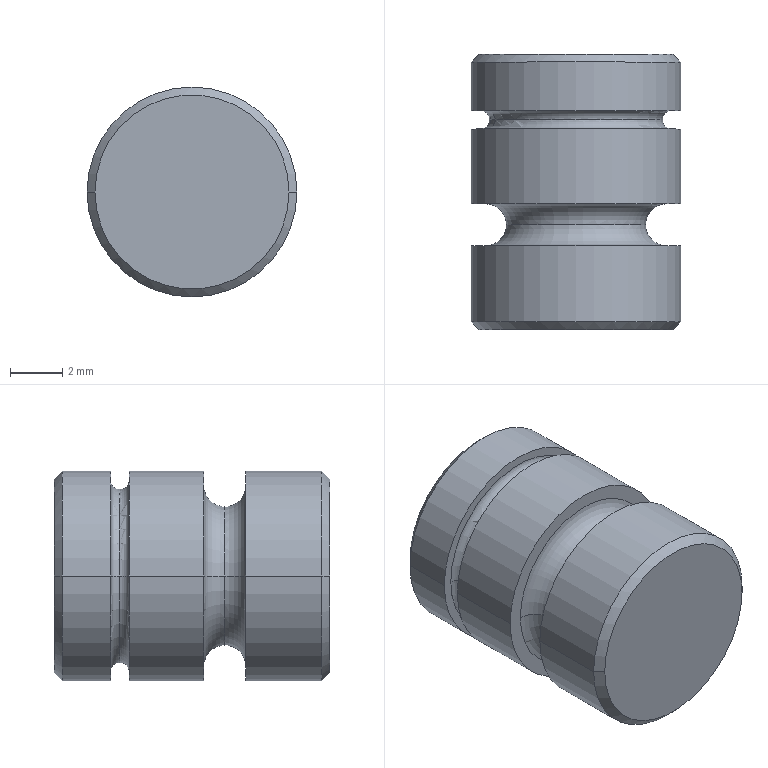Part | Creo | 1 solid | 27 faces | box 8 x 10.5 x 8 mm | volume 445.026 mm3 | cylinder 8 | torus 8 | plane 7 | cone 4 | commonest cylinder face diameters 8 x6 6.2 x2
STEP:
#1=CARTESIAN_POINT('',(0.,0.,0.));
#2=DIRECTION('',(0.,0.,1.));
#3=DIRECTION('',(1.,0.,0.));
#4=AXIS2_PLACEMENT_3D('',#1,#2,#3);
#5=CARTESIAN_POINT('',(59.,47.3,60.91));
#6=VERTEX_POINT('',#5);
#7=CARTESIAN_POINT('',(51.,47.3,60.91));
#8=VERTEX_POINT('',#7);
#9=CARTESIAN_POINT('',(55.,47.3,60.91));
#10=DIRECTION('',(0.,-1.,0.));
#11=DIRECTION('',(1.,0.,0.));
#12=AXIS2_PLACEMENT_3D('',#9,#10,#11);
#13=CIRCLE('',#12,4.);
#14=EDGE_CURVE('',#6,#8,#13,.T.);
#15=ORIENTED_EDGE('',*,*,#14,.T.);
#16=CARTESIAN_POINT('',(51.,50.15,60.91));
#17=VERTEX_POINT('',#16);
#18=CARTESIAN_POINT('',(51.,47.3,60.91));
#19=DIRECTION('',(0.,1.,0.));
#20=VECTOR('',#19,2.85);
#21=LINE('',#18,#20);
#22=EDGE_CURVE('',#8,#17,#21,.T.);
#23=ORIENTED_EDGE('',*,*,#22,.T.);
#24=CARTESIAN_POINT('',(59.,50.15,60.91));
#25=VERTEX_POINT('',#24);
#26=CARTESIAN_POINT('',(55.,50.15,60.91));
#27=DIRECTION('',(0.,1.,0.));
#28=DIRECTION('',(-1.,0.,0.));
#29=AXIS2_PLACEMENT_3D('',#26,#27,#28);
#30=CIRCLE('',#29,4.);
#31=EDGE_CURVE('',#17,#25,#30,.T.);
#32=ORIENTED_EDGE('',*,*,#31,.T.);
#33=CARTESIAN_POINT('',(59.,47.3,60.91));
#34=DIRECTION('',(0.,1.,0.));
#35=VECTOR('',#34,2.85);
#36=LINE('',#33,#35);
#37=EDGE_CURVE('',#6,#25,#36,.T.);
#38=ORIENTED_EDGE('',*,*,#37,.F.);
#39=EDGE_LOOP('',(#15,#23,#32,#38));
#40=FACE_OUTER_BOUND('',#39,.F.);
#41=CARTESIAN_POINT('',(55.,42.5,60.91));
#42=DIRECTION('',(0.,1.,0.));
#43=DIRECTION('',(-1.,0.,0.));
#44=AXIS2_PLACEMENT_3D('',#41,#42,#43);
#45=CYLINDRICAL_SURFACE('',#44,4.);
#46=ADVANCED_FACE('',(#40),#45,.T.);
#47=ORIENTED_EDGE('',*,*,#14,.F.);
#48=CARTESIAN_POINT('',(55.,47.3,60.91));
#49=DIRECTION('',(0.,-1.,0.));
#50=DIRECTION('',(-1.,0.,0.));
#51=AXIS2_PLACEMENT_3D('',#48,#49,#50);
#52=CIRCLE('',#51,4.);
#53=EDGE_CURVE('',#8,#6,#52,.T.);
#54=ORIENTED_EDGE('',*,*,#53,.F.);
#55=EDGE_LOOP('',(#47,#54));
#56=FACE_OUTER_BOUND('',#55,.F.);
#57=CARTESIAN_POINT('',(51.55,47.3,60.91));
#58=VERTEX_POINT('',#57);
#59=CARTESIAN_POINT('',(58.45,47.3,60.91));
#60=VERTEX_POINT('',#59);
#61=CARTESIAN_POINT('',(55.,47.3,60.91));
#62=DIRECTION('',(0.,1.,0.));
#63=DIRECTION('',(-1.,0.,0.));
#64=AXIS2_PLACEMENT_3D('',#61,#62,#63);
#65=CIRCLE('',#64,3.45);
#66=EDGE_CURVE('',#58,#60,#65,.T.);
#67=ORIENTED_EDGE('',*,*,#66,.F.);
#68=CARTESIAN_POINT('',(55.,47.3,60.91));
#69=DIRECTION('',(0.,1.,0.));
#70=DIRECTION('',(1.,0.,0.));
#71=AXIS2_PLACEMENT_3D('',#68,#69,#70);
#72=CIRCLE('',#71,3.45);
#73=EDGE_CURVE('',#60,#58,#72,.T.);
#74=ORIENTED_EDGE('',*,*,#73,.F.);
#75=EDGE_LOOP('',(#67,#74));
#76=FACE_BOUND('',#75,.F.);
#77=CARTESIAN_POINT('',(63.45,47.3,60.91));
#78=DIRECTION('',(0.,-1.,0.));
#79=DIRECTION('',(1.,0.,0.));
#80=AXIS2_PLACEMENT_3D('',#77,#78,#79);
#81=PLANE('',#80);
#82=ADVANCED_FACE('',(#56,#76),#81,.T.);
#83=ORIENTED_EDGE('',*,*,#66,.T.);
#84=CARTESIAN_POINT('',(57.65,46.5,60.91));
#85=VERTEX_POINT('',#84);
#86=CARTESIAN_POINT('',(58.45,46.5,60.91));
#87=DIRECTION('',(0.,0.,1.));
#88=DIRECTION('',(0.,1.,0.));
#89=AXIS2_PLACEMENT_3D('',#86,#87,#88);
#90=CIRCLE('',#89,0.8);
#91=EDGE_CURVE('',#60,#85,#90,.T.);
#92=ORIENTED_EDGE('',*,*,#91,.T.);
#93=CARTESIAN_POINT('',(52.35,46.5,60.91));
#94=VERTEX_POINT('',#93);
#95=CARTESIAN_POINT('',(55.,46.5,60.91));
#96=DIRECTION('',(0.,1.,0.));
#97=DIRECTION('',(-1.,0.,0.));
#98=AXIS2_PLACEMENT_3D('',#95,#96,#97);
#99=CIRCLE('',#98,2.65);
#100=EDGE_CURVE('',#94,#85,#99,.T.);
#101=ORIENTED_EDGE('',*,*,#100,.F.);
#102=CARTESIAN_POINT('',(51.55,46.5,60.91));
#103=DIRECTION('',(0.,0.,-1.));
#104=DIRECTION('',(0.,1.,0.));
#105=AXIS2_PLACEMENT_3D('',#102,#103,#104);
#106=CIRCLE('',#105,0.8);
#107=EDGE_CURVE('',#58,#94,#106,.T.);
#108=ORIENTED_EDGE('',*,*,#107,.F.);
#109=EDGE_LOOP('',(#83,#92,#101,#108));
#110=FACE_OUTER_BOUND('',#109,.F.);
#111=CARTESIAN_POINT('',(55.,46.5,60.91));
#112=DIRECTION('',(0.,1.,0.));
#113=DIRECTION('',(-1.,0.,0.));
#114=AXIS2_PLACEMENT_3D('',#111,#112,#113);
#115=TOROIDAL_SURFACE('',#114,3.45,0.8);
#116=ADVANCED_FACE('',(#110),#115,.F.);
#117=ORIENTED_EDGE('',*,*,#73,.T.);
#118=ORIENTED_EDGE('',*,*,#107,.T.);
#119=CARTESIAN_POINT('',(55.,46.5,60.91));
#120=DIRECTION('',(0.,1.,0.));
#121=DIRECTION('',(1.,0.,0.));
#122=AXIS2_PLACEMENT_3D('',#119,#120,#121);
#123=CIRCLE('',#122,2.65);
#124=EDGE_CURVE('',#85,#94,#123,.T.);
#125=ORIENTED_EDGE('',*,*,#124,.F.);
#126=ORIENTED_EDGE('',*,*,#91,.F.);
#127=EDGE_LOOP('',(#117,#118,#125,#126));
#128=FACE_OUTER_BOUND('',#127,.F.);
#129=CARTESIAN_POINT('',(55.,46.5,60.91));
#130=DIRECTION('',(0.,1.,0.));
#131=DIRECTION('',(-1.,0.,0.));
#132=AXIS2_PLACEMENT_3D('',#129,#130,#131);
#133=TOROIDAL_SURFACE('',#132,3.45,0.8);
#134=ADVANCED_FACE('',(#128),#133,.F.);
#135=CARTESIAN_POINT('',(51.55,45.7,60.91));
#136=VERTEX_POINT('',#135);
#137=CARTESIAN_POINT('',(58.45,45.7,60.91));
#138=VERTEX_POINT('',#137);
#139=CARTESIAN_POINT('',(55.,45.7,60.91));
#140=DIRECTION('',(0.,-1.,0.));
#141=DIRECTION('',(-1.,0.,0.));
#142=AXIS2_PLACEMENT_3D('',#139,#140,#141);
#143=CIRCLE('',#142,3.45);
#144=EDGE_CURVE('',#136,#138,#143,.T.);
#145=ORIENTED_EDGE('',*,*,#144,.T.);
#146=CARTESIAN_POINT('',(58.45,46.5,60.91));
#147=DIRECTION('',(0.,0.,1.));
#148=DIRECTION('',(-1.,0.,0.));
#149=AXIS2_PLACEMENT_3D('',#146,#147,#148);
#150=CIRCLE('',#149,0.8);
#151=EDGE_CURVE('',#85,#138,#150,.T.);
#152=ORIENTED_EDGE('',*,*,#151,.F.);
#153=ORIENTED_EDGE('',*,*,#124,.T.);
#154=CARTESIAN_POINT('',(51.55,46.5,60.91));
#155=DIRECTION('',(0.,0.,-1.));
#156=DIRECTION('',(1.,0.,0.));
#157=AXIS2_PLACEMENT_3D('',#154,#155,#156);
#158=CIRCLE('',#157,0.8);
#159=EDGE_CURVE('',#94,#136,#158,.T.);
#160=ORIENTED_EDGE('',*,*,#159,.T.);
#161=EDGE_LOOP('',(#145,#152,#153,#160));
#162=FACE_OUTER_BOUND('',#161,.F.);
#163=CARTESIAN_POINT('',(55.,46.5,60.91));
#164=DIRECTION('',(0.,1.,0.));
#165=DIRECTION('',(-1.,0.,0.));
#166=AXIS2_PLACEMENT_3D('',#163,#164,#165);
#167=TOROIDAL_SURFACE('',#166,3.45,0.8);
#168=ADVANCED_FACE('',(#162),#167,.F.);
#169=CARTESIAN_POINT('',(51.,45.7,60.91));
#170=VERTEX_POINT('',#169);
#171=CARTESIAN_POINT('',(59.,45.7,60.91));
#172=VERTEX_POINT('',#171);
#173=CARTESIAN_POINT('',(55.,45.7,60.91));
#174=DIRECTION('',(0.,1.,0.));
#175=DIRECTION('',(-1.,0.,0.));
#176=AXIS2_PLACEMENT_3D('',#173,#174,#175);
#177=CIRCLE('',#176,4.);
#178=EDGE_CURVE('',#170,#172,#177,.T.);
#179=ORIENTED_EDGE('',*,*,#178,.F.);
#180=CARTESIAN_POINT('',(55.,45.7,60.91));
#181=DIRECTION('',(0.,1.,0.));
#182=DIRECTION('',(1.,0.,0.));
#183=AXIS2_PLACEMENT_3D('',#180,#181,#182);
#184=CIRCLE('',#183,4.);
#185=EDGE_CURVE('',#172,#170,#184,.T.);
#186=ORIENTED_EDGE('',*,*,#185,.F.);
#187=EDGE_LOOP('',(#179,#186));
#188=FACE_OUTER_BOUND('',#187,.F.);
#189=ORIENTED_EDGE('',*,*,#144,.F.);
#190=CARTESIAN_POINT('',(55.,45.7,60.91));
#191=DIRECTION('',(0.,-1.,0.));
#192=DIRECTION('',(1.,0.,0.));
#193=AXIS2_PLACEMENT_3D('',#190,#191,#192);
#194=CIRCLE('',#193,3.45);
#195=EDGE_CURVE('',#138,#136,#194,.T.);
#196=ORIENTED_EDGE('',*,*,#195,.F.);
#197=EDGE_LOOP('',(#189,#196));
#198=FACE_BOUND('',#197,.F.);
#199=CARTESIAN_POINT('',(58.45,45.7,60.91));
#200=DIRECTION('',(0.,1.,0.));
#201=DIRECTION('',(-1.,0.,0.));
#202=AXIS2_PLACEMENT_3D('',#199,#200,#201);
#203=PLANE('',#202);
#204=ADVANCED_FACE('',(#188,#198),#203,.T.);
#205=ORIENTED_EDGE('',*,*,#195,.T.);
#206=ORIENTED_EDGE('',*,*,#159,.F.);
#207=ORIENTED_EDGE('',*,*,#100,.T.);
#208=ORIENTED_EDGE('',*,*,#151,.T.);
#209=EDGE_LOOP('',(#205,#206,#207,#208));
#210=FACE_OUTER_BOUND('',#209,.F.);
#211=CARTESIAN_POINT('',(55.,46.5,60.91));
#212=DIRECTION('',(0.,1.,0.));
#213=DIRECTION('',(-1.,0.,0.));
#214=AXIS2_PLACEMENT_3D('',#211,#212,#213);
#215=TOROIDAL_SURFACE('',#214,3.45,0.8);
#216=ADVANCED_FACE('',(#210),#215,.F.);
#217=CARTESIAN_POINT('',(59.,42.8,60.91));
#218=VERTEX_POINT('',#217);
#219=CARTESIAN_POINT('',(51.,42.8,60.91));
#220=VERTEX_POINT('',#219);
#221=CARTESIAN_POINT('',(55.,42.8,60.91));
#222=DIRECTION('',(0.,-1.,0.));
#223=DIRECTION('',(1.,0.,0.));
#224=AXIS2_PLACEMENT_3D('',#221,#222,#223);
#225=CIRCLE('',#224,4.);
#226=EDGE_CURVE('',#218,#220,#225,.T.);
#227=ORIENTED_EDGE('',*,*,#226,.T.);
#228=CARTESIAN_POINT('',(51.,42.8,60.91));
#229=DIRECTION('',(0.,1.,0.));
#230=VECTOR('',#229,2.9);
#231=LINE('',#228,#230);
#232=EDGE_CURVE('',#220,#170,#231,.T.);
#233=ORIENTED_EDGE('',*,*,#232,.T.);
#234=ORIENTED_EDGE('',*,*,#178,.T.);
#235=CARTESIAN_POINT('',(59.,42.8,60.91));
#236=DIRECTION('',(0.,1.,0.));
#237=VECTOR('',#236,2.9);
#238=LINE('',#235,#237);
#239=EDGE_CURVE('',#218,#172,#238,.T.);
#240=ORIENTED_EDGE('',*,*,#239,.F.);
#241=EDGE_LOOP('',(#227,#233,#234,#240));
#242=FACE_OUTER_BOUND('',#241,.F.);
#243=CARTESIAN_POINT('',(55.,42.5,60.91));
#244=DIRECTION('',(0.,1.,0.));
#245=DIRECTION('',(-1.,0.,0.));
#246=AXIS2_PLACEMENT_3D('',#243,#244,#245);
#247=CYLINDRICAL_SURFACE('',#246,4.);
#248=ADVANCED_FACE('',(#242),#247,.T.);
#249=ORIENTED_EDGE('',*,*,#226,.F.);
#250=CARTESIAN_POINT('',(58.7,42.5,60.91));
#251=VERTEX_POINT('',#250);
#252=CARTESIAN_POINT('',(58.7,42.5,60.91));
#253=DIRECTION('',(0.7071,0.7071,0.));
#254=VECTOR('',#253,0.4243);
#255=LINE('',#252,#254);
#256=EDGE_CURVE('',#251,#218,#255,.T.);
#257=ORIENTED_EDGE('',*,*,#256,.F.);
#258=CARTESIAN_POINT('',(51.3,42.5,60.91));
#259=VERTEX_POINT('',#258);
#260=CARTESIAN_POINT('',(55.,42.5,60.91));
#261=DIRECTION('',(0.,-1.,0.));
#262=DIRECTION('',(1.,0.,0.));
#263=AXIS2_PLACEMENT_3D('',#260,#261,#262);
#264=CIRCLE('',#263,3.7);
#265=EDGE_CURVE('',#251,#259,#264,.T.);
#266=ORIENTED_EDGE('',*,*,#265,.T.);
#267=CARTESIAN_POINT('',(51.3,42.5,60.91));
#268=DIRECTION('',(-0.7071,0.7071,0.));
#269=VECTOR('',#268,0.4243);
#270=LINE('',#267,#269);
#271=EDGE_CURVE('',#259,#220,#270,.T.);
#272=ORIENTED_EDGE('',*,*,#271,.T.);
#273=EDGE_LOOP('',(#249,#257,#266,#272));
#274=FACE_OUTER_BOUND('',#273,.F.);
#275=CARTESIAN_POINT('',(55.,42.65,60.91));
#276=DIRECTION('',(0.,1.,0.));
#277=DIRECTION('',(-1.,0.,0.));
#278=AXIS2_PLACEMENT_3D('',#275,#276,#277);
#279=CONICAL_SURFACE('',#278,3.85,45.);
#280=ADVANCED_FACE('',(#274),#279,.T.);
#281=CARTESIAN_POINT('',(55.,42.8,60.91));
#282=DIRECTION('',(0.,-1.,0.));
#283=DIRECTION('',(-1.,0.,0.));
#284=AXIS2_PLACEMENT_3D('',#281,#282,#283);
#285=CIRCLE('',#284,4.);
#286=EDGE_CURVE('',#220,#218,#285,.T.);
#287=ORIENTED_EDGE('',*,*,#286,.F.);
#288=ORIENTED_EDGE('',*,*,#271,.F.);
#289=CARTESIAN_POINT('',(55.,42.5,60.91));
#290=DIRECTION('',(0.,-1.,0.));
#291=DIRECTION('',(-1.,0.,0.));
#292=AXIS2_PLACEMENT_3D('',#289,#290,#291);
#293=CIRCLE('',#292,3.7);
#294=EDGE_CURVE('',#259,#251,#293,.T.);
#295=ORIENTED_EDGE('',*,*,#294,.T.);
#296=ORIENTED_EDGE('',*,*,#256,.T.);
#297=EDGE_LOOP('',(#287,#288,#295,#296));
#298=FACE_OUTER_BOUND('',#297,.F.);
#299=CARTESIAN_POINT('',(55.,42.65,60.91));
#300=DIRECTION('',(0.,1.,0.));
#301=DIRECTION('',(-1.,0.,0.));
#302=AXIS2_PLACEMENT_3D('',#299,#300,#301);
#303=CONICAL_SURFACE('',#302,3.85,45.);
#304=ADVANCED_FACE('',(#298),#303,.T.);
#305=ORIENTED_EDGE('',*,*,#286,.T.);
#306=ORIENTED_EDGE('',*,*,#239,.T.);
#307=ORIENTED_EDGE('',*,*,#185,.T.);
#308=ORIENTED_EDGE('',*,*,#232,.F.);
#309=EDGE_LOOP('',(#305,#306,#307,#308));
#310=FACE_OUTER_BOUND('',#309,.F.);
#311=CARTESIAN_POINT('',(55.,42.5,60.91));
#312=DIRECTION('',(0.,1.,0.));
#313=DIRECTION('',(-1.,0.,0.));
#314=AXIS2_PLACEMENT_3D('',#311,#312,#313);
#315=CYLINDRICAL_SURFACE('',#314,4.);
#316=ADVANCED_FACE('',(#310),#315,.T.);
#317=ORIENTED_EDGE('',*,*,#265,.F.);
#318=ORIENTED_EDGE('',*,*,#294,.F.);
#319=EDGE_LOOP('',(#317,#318));
#320=FACE_OUTER_BOUND('',#319,.F.);
#321=CARTESIAN_POINT('',(55.,42.5,60.91));
#322=DIRECTION('',(0.,-1.,0.));
#323=DIRECTION('',(1.,0.,0.));
#324=AXIS2_PLACEMENT_3D('',#321,#322,#323);
#325=PLANE('',#324);
#326=ADVANCED_FACE('',(#320),#325,.T.);
#327=ORIENTED_EDGE('',*,*,#53,.T.);
#328=ORIENTED_EDGE('',*,*,#37,.T.);
#329=CARTESIAN_POINT('',(55.,50.15,60.91));
#330=DIRECTION('',(0.,1.,0.));
#331=DIRECTION('',(1.,0.,0.));
#332=AXIS2_PLACEMENT_3D('',#329,#330,#331);
#333=CIRCLE('',#332,4.);
#334=EDGE_CURVE('',#25,#17,#333,.T.);
#335=ORIENTED_EDGE('',*,*,#334,.T.);
#336=ORIENTED_EDGE('',*,*,#22,.F.);
#337=EDGE_LOOP('',(#327,#328,#335,#336));
#338=FACE_OUTER_BOUND('',#337,.F.);
#339=CARTESIAN_POINT('',(55.,42.5,60.91));
#340=DIRECTION('',(0.,1.,0.));
#341=DIRECTION('',(-1.,0.,0.));
#342=AXIS2_PLACEMENT_3D('',#339,#340,#341);
#343=CYLINDRICAL_SURFACE('',#342,4.);
#344=ADVANCED_FACE('',(#338),#343,.T.);
#345=ORIENTED_EDGE('',*,*,#31,.F.);
#346=ORIENTED_EDGE('',*,*,#334,.F.);
#347=EDGE_LOOP('',(#345,#346));
#348=FACE_OUTER_BOUND('',#347,.F.);
#349=CARTESIAN_POINT('',(51.35,50.15,60.91));
#350=VERTEX_POINT('',#349);
#351=CARTESIAN_POINT('',(58.65,50.15,60.91));
#352=VERTEX_POINT('',#351);
#353=CARTESIAN_POINT('',(55.,50.15,60.91));
#354=DIRECTION('',(0.,-1.,0.));
#355=DIRECTION('',(-1.,0.,0.));
#356=AXIS2_PLACEMENT_3D('',#353,#354,#355);
#357=CIRCLE('',#356,3.65);
#358=EDGE_CURVE('',#350,#352,#357,.T.);
#359=ORIENTED_EDGE('',*,*,#358,.F.);
#360=CARTESIAN_POINT('',(55.,50.15,60.91));
#361=DIRECTION('',(0.,-1.,0.));
#362=DIRECTION('',(1.,0.,0.));
#363=AXIS2_PLACEMENT_3D('',#360,#361,#362);
#364=CIRCLE('',#363,3.65);
#365=EDGE_CURVE('',#352,#350,#364,.T.);
#366=ORIENTED_EDGE('',*,*,#365,.F.);
#367=EDGE_LOOP('',(#359,#366));
#368=FACE_BOUND('',#367,.F.);
#369=CARTESIAN_POINT('',(58.65,50.15,60.91));
#370=DIRECTION('',(0.,1.,0.));
#371=DIRECTION('',(-1.,0.,0.));
#372=AXIS2_PLACEMENT_3D('',#369,#370,#371);
#373=PLANE('',#372);
#374=ADVANCED_FACE('',(#348,#368),#373,.T.);
#375=ORIENTED_EDGE('',*,*,#358,.T.);
#376=CARTESIAN_POINT('',(58.3,50.5,60.91));
#377=VERTEX_POINT('',#376);
#378=CARTESIAN_POINT('',(58.65,50.5,60.91));
#379=DIRECTION('',(0.,0.,1.));
#380=DIRECTION('',(-1.,0.,0.));
#381=AXIS2_PLACEMENT_3D('',#378,#379,#380);
#382=CIRCLE('',#381,0.35);
#383=EDGE_CURVE('',#377,#352,#382,.T.);
#384=ORIENTED_EDGE('',*,*,#383,.F.);
#385=CARTESIAN_POINT('',(51.7,50.5,60.91));
#386=VERTEX_POINT('',#385);
#387=CARTESIAN_POINT('',(55.,50.5,60.91));
#388=DIRECTION('',(0.,1.,0.));
#389=DIRECTION('',(1.,0.,0.));
#390=AXIS2_PLACEMENT_3D('',#387,#388,#389);
#391=CIRCLE('',#390,3.3);
#392=EDGE_CURVE('',#377,#386,#391,.T.);
#393=ORIENTED_EDGE('',*,*,#392,.T.);
#394=CARTESIAN_POINT('',(51.35,50.5,60.91));
#395=DIRECTION('',(0.,0.,-1.));
#396=DIRECTION('',(1.,0.,0.));
#397=AXIS2_PLACEMENT_3D('',#394,#395,#396);
#398=CIRCLE('',#397,0.35);
#399=EDGE_CURVE('',#386,#350,#398,.T.);
#400=ORIENTED_EDGE('',*,*,#399,.T.);
#401=EDGE_LOOP('',(#375,#384,#393,#400));
#402=FACE_OUTER_BOUND('',#401,.F.);
#403=CARTESIAN_POINT('',(55.,50.5,60.91));
#404=DIRECTION('',(0.,1.,0.));
#405=DIRECTION('',(-1.,0.,0.));
#406=AXIS2_PLACEMENT_3D('',#403,#404,#405);
#407=TOROIDAL_SURFACE('',#406,3.65,0.35);
#408=ADVANCED_FACE('',(#402),#407,.F.);
#409=ORIENTED_EDGE('',*,*,#365,.T.);
#410=ORIENTED_EDGE('',*,*,#399,.F.);
#411=CARTESIAN_POINT('',(55.,50.5,60.91));
#412=DIRECTION('',(0.,1.,0.));
#413=DIRECTION('',(-1.,0.,0.));
#414=AXIS2_PLACEMENT_3D('',#411,#412,#413);
#415=CIRCLE('',#414,3.3);
#416=EDGE_CURVE('',#386,#377,#415,.T.);
#417=ORIENTED_EDGE('',*,*,#416,.T.);
#418=ORIENTED_EDGE('',*,*,#383,.T.);
#419=EDGE_LOOP('',(#409,#410,#417,#418));
#420=FACE_OUTER_BOUND('',#419,.F.);
#421=CARTESIAN_POINT('',(55.,50.5,60.91));
#422=DIRECTION('',(0.,1.,0.));
#423=DIRECTION('',(-1.,0.,0.));
#424=AXIS2_PLACEMENT_3D('',#421,#422,#423);
#425=TOROIDAL_SURFACE('',#424,3.65,0.35);
#426=ADVANCED_FACE('',(#420),#425,.F.);
#427=CARTESIAN_POINT('',(51.35,50.85,60.91));
#428=VERTEX_POINT('',#427);
#429=CARTESIAN_POINT('',(58.65,50.85,60.91));
#430=VERTEX_POINT('',#429);
#431=CARTESIAN_POINT('',(55.,50.85,60.91));
#432=DIRECTION('',(0.,1.,0.));
#433=DIRECTION('',(-1.,0.,0.));
#434=AXIS2_PLACEMENT_3D('',#431,#432,#433);
#435=CIRCLE('',#434,3.65);
#436=EDGE_CURVE('',#428,#430,#435,.T.);
#437=ORIENTED_EDGE('',*,*,#436,.T.);
#438=CARTESIAN_POINT('',(58.65,50.5,60.91));
#439=DIRECTION('',(0.,0.,1.));
#440=DIRECTION('',(0.,1.,0.));
#441=AXIS2_PLACEMENT_3D('',#438,#439,#440);
#442=CIRCLE('',#441,0.35);
#443=EDGE_CURVE('',#430,#377,#442,.T.);
#444=ORIENTED_EDGE('',*,*,#443,.T.);
#445=ORIENTED_EDGE('',*,*,#416,.F.);
#446=CARTESIAN_POINT('',(51.35,50.5,60.91));
#447=DIRECTION('',(0.,0.,-1.));
#448=DIRECTION('',(0.,1.,0.));
#449=AXIS2_PLACEMENT_3D('',#446,#447,#448);
#450=CIRCLE('',#449,0.35);
#451=EDGE_CURVE('',#428,#386,#450,.T.);
#452=ORIENTED_EDGE('',*,*,#451,.F.);
#453=EDGE_LOOP('',(#437,#444,#445,#452));
#454=FACE_OUTER_BOUND('',#453,.F.);
#455=CARTESIAN_POINT('',(55.,50.5,60.91));
#456=DIRECTION('',(0.,1.,0.));
#457=DIRECTION('',(-1.,0.,0.));
#458=AXIS2_PLACEMENT_3D('',#455,#456,#457);
#459=TOROIDAL_SURFACE('',#458,3.65,0.35);
#460=ADVANCED_FACE('',(#454),#459,.F.);
#461=CARTESIAN_POINT('',(59.,50.85,60.91));
#462=VERTEX_POINT('',#461);
#463=CARTESIAN_POINT('',(51.,50.85,60.91));
#464=VERTEX_POINT('',#463);
#465=CARTESIAN_POINT('',(55.,50.85,60.91));
#466=DIRECTION('',(0.,-1.,0.));
#467=DIRECTION('',(1.,0.,0.));
#468=AXIS2_PLACEMENT_3D('',#465,#466,#467);
#469=CIRCLE('',#468,4.);
#470=EDGE_CURVE('',#462,#464,#469,.T.);
#471=ORIENTED_EDGE('',*,*,#470,.F.);
#472=CARTESIAN_POINT('',(55.,50.85,60.91));
#473=DIRECTION('',(0.,-1.,0.));
#474=DIRECTION('',(-1.,0.,0.));
#475=AXIS2_PLACEMENT_3D('',#472,#473,#474);
#476=CIRCLE('',#475,4.);
#477=EDGE_CURVE('',#464,#462,#476,.T.);
#478=ORIENTED_EDGE('',*,*,#477,.F.);
#479=EDGE_LOOP('',(#471,#478));
#480=FACE_OUTER_BOUND('',#479,.F.);
#481=ORIENTED_EDGE('',*,*,#436,.F.);
#482=CARTESIAN_POINT('',(55.,50.85,60.91));
#483=DIRECTION('',(0.,1.,0.));
#484=DIRECTION('',(1.,0.,0.));
#485=AXIS2_PLACEMENT_3D('',#482,#483,#484);
#486=CIRCLE('',#485,3.65);
#487=EDGE_CURVE('',#430,#428,#486,.T.);
#488=ORIENTED_EDGE('',*,*,#487,.F.);
#489=EDGE_LOOP('',(#481,#488));
#490=FACE_BOUND('',#489,.F.);
#491=CARTESIAN_POINT('',(63.65,50.85,60.91));
#492=DIRECTION('',(0.,-1.,0.));
#493=DIRECTION('',(1.,0.,0.));
#494=AXIS2_PLACEMENT_3D('',#491,#492,#493);
#495=PLANE('',#494);
#496=ADVANCED_FACE('',(#480,#490),#495,.T.);
#497=ORIENTED_EDGE('',*,*,#487,.T.);
#498=ORIENTED_EDGE('',*,*,#451,.T.);
#499=ORIENTED_EDGE('',*,*,#392,.F.);
#500=ORIENTED_EDGE('',*,*,#443,.F.);
#501=EDGE_LOOP('',(#497,#498,#499,#500));
#502=FACE_OUTER_BOUND('',#501,.F.);
#503=CARTESIAN_POINT('',(55.,50.5,60.91));
#504=DIRECTION('',(0.,1.,0.));
#505=DIRECTION('',(-1.,0.,0.));
#506=AXIS2_PLACEMENT_3D('',#503,#504,#505);
#507=TOROIDAL_SURFACE('',#506,3.65,0.35);
#508=ADVANCED_FACE('',(#502),#507,.F.);
#509=CARTESIAN_POINT('',(51.,52.7,60.91));
#510=VERTEX_POINT('',#509);
#511=CARTESIAN_POINT('',(59.,52.7,60.91));
#512=VERTEX_POINT('',#511);
#513=CARTESIAN_POINT('',(55.,52.7,60.91));
#514=DIRECTION('',(0.,1.,0.));
#515=DIRECTION('',(-1.,0.,0.));
#516=AXIS2_PLACEMENT_3D('',#513,#514,#515);
#517=CIRCLE('',#516,4.);
#518=EDGE_CURVE('',#510,#512,#517,.T.);
#519=ORIENTED_EDGE('',*,*,#518,.T.);
#520=CARTESIAN_POINT('',(59.,50.85,60.91));
#521=DIRECTION('',(0.,1.,0.));
#522=VECTOR('',#521,1.85);
#523=LINE('',#520,#522);
#524=EDGE_CURVE('',#462,#512,#523,.T.);
#525=ORIENTED_EDGE('',*,*,#524,.F.);
#526=ORIENTED_EDGE('',*,*,#470,.T.);
#527=CARTESIAN_POINT('',(51.,50.85,60.91));
#528=DIRECTION('',(0.,1.,0.));
#529=VECTOR('',#528,1.85);
#530=LINE('',#527,#529);
#531=EDGE_CURVE('',#464,#510,#530,.T.);
#532=ORIENTED_EDGE('',*,*,#531,.T.);
#533=EDGE_LOOP('',(#519,#525,#526,#532));
#534=FACE_OUTER_BOUND('',#533,.F.);
#535=CARTESIAN_POINT('',(55.,42.5,60.91));
#536=DIRECTION('',(0.,1.,0.));
#537=DIRECTION('',(-1.,0.,0.));
#538=AXIS2_PLACEMENT_3D('',#535,#536,#537);
#539=CYLINDRICAL_SURFACE('',#538,4.);
#540=ADVANCED_FACE('',(#534),#539,.T.);
#541=CARTESIAN_POINT('',(51.3,53.,60.91));
#542=VERTEX_POINT('',#541);
#543=CARTESIAN_POINT('',(58.7,53.,60.91));
#544=VERTEX_POINT('',#543);
#545=CARTESIAN_POINT('',(55.,53.,60.91));
#546=DIRECTION('',(0.,1.,0.));
#547=DIRECTION('',(-1.,0.,0.));
#548=AXIS2_PLACEMENT_3D('',#545,#546,#547);
#549=CIRCLE('',#548,3.7);
#550=EDGE_CURVE('',#542,#544,#549,.T.);
#551=ORIENTED_EDGE('',*,*,#550,.T.);
#552=CARTESIAN_POINT('',(58.7,53.,60.91));
#553=DIRECTION('',(0.7071,-0.7071,0.));
#554=VECTOR('',#553,0.4243);
#555=LINE('',#552,#554);
#556=EDGE_CURVE('',#544,#512,#555,.T.);
#557=ORIENTED_EDGE('',*,*,#556,.T.);
#558=ORIENTED_EDGE('',*,*,#518,.F.);
#559=CARTESIAN_POINT('',(51.3,53.,60.91));
#560=DIRECTION('',(-0.7071,-0.7071,0.));
#561=VECTOR('',#560,0.4243);
#562=LINE('',#559,#561);
#563=EDGE_CURVE('',#542,#510,#562,.T.);
#564=ORIENTED_EDGE('',*,*,#563,.F.);
#565=EDGE_LOOP('',(#551,#557,#558,#564));
#566=FACE_OUTER_BOUND('',#565,.F.);
#567=CARTESIAN_POINT('',(55.,52.85,60.91));
#568=DIRECTION('',(0.,-1.,0.));
#569=DIRECTION('',(1.,0.,0.));
#570=AXIS2_PLACEMENT_3D('',#567,#568,#569);
#571=CONICAL_SURFACE('',#570,3.85,45.);
#572=ADVANCED_FACE('',(#566),#571,.T.);
#573=CARTESIAN_POINT('',(55.,53.,60.91));
#574=DIRECTION('',(0.,1.,0.));
#575=DIRECTION('',(1.,0.,0.));
#576=AXIS2_PLACEMENT_3D('',#573,#574,#575);
#577=CIRCLE('',#576,3.7);
#578=EDGE_CURVE('',#544,#542,#577,.T.);
#579=ORIENTED_EDGE('',*,*,#578,.F.);
#580=ORIENTED_EDGE('',*,*,#550,.F.);
#581=EDGE_LOOP('',(#579,#580));
#582=FACE_OUTER_BOUND('',#581,.F.);
#583=CARTESIAN_POINT('',(55.,53.,64.01));
#584=VERTEX_POINT('',#583);
#585=CARTESIAN_POINT('',(51.9,53.,60.91));
#586=VERTEX_POINT('',#585);
#587=CARTESIAN_POINT('',(55.,53.,60.91));
#588=DIRECTION('',(0.,-1.,0.));
#589=DIRECTION('',(0.,0.,1.));
#590=AXIS2_PLACEMENT_3D('',#587,#588,#589);
#591=CIRCLE('',#590,3.1);
#592=EDGE_CURVE('',#584,#586,#591,.T.);
#593=ORIENTED_EDGE('',*,*,#592,.F.);
#594=CARTESIAN_POINT('',(58.1,53.,60.91));
#595=VERTEX_POINT('',#594);
#596=CARTESIAN_POINT('',(55.,53.,60.91));
#597=DIRECTION('',(0.,-1.,0.));
#598=DIRECTION('',(1.,0.,0.));
#599=AXIS2_PLACEMENT_3D('',#596,#597,#598);
#600=CIRCLE('',#599,3.1);
#601=EDGE_CURVE('',#595,#584,#600,.T.);
#602=ORIENTED_EDGE('',*,*,#601,.F.);
#603=CARTESIAN_POINT('',(55.,53.,57.81));
#604=VERTEX_POINT('',#603);
#605=CARTESIAN_POINT('',(55.,53.,60.91));
#606=DIRECTION('',(0.,-1.,0.));
#607=DIRECTION('',(0.,0.,-1.));
#608=AXIS2_PLACEMENT_3D('',#605,#606,#607);
#609=CIRCLE('',#608,3.1);
#610=EDGE_CURVE('',#604,#595,#609,.T.);
#611=ORIENTED_EDGE('',*,*,#610,.F.);
#612=CARTESIAN_POINT('',(55.,53.,60.91));
#613=DIRECTION('',(0.,-1.,0.));
#614=DIRECTION('',(-1.,0.,0.));
#615=AXIS2_PLACEMENT_3D('',#612,#613,#614);
#616=CIRCLE('',#615,3.1);
#617=EDGE_CURVE('',#586,#604,#616,.T.);
#618=ORIENTED_EDGE('',*,*,#617,.F.);
#619=EDGE_LOOP('',(#593,#602,#611,#618));
#620=FACE_BOUND('',#619,.F.);
#621=CARTESIAN_POINT('',(55.,53.,60.91));
#622=DIRECTION('',(0.,-1.,0.));
#623=DIRECTION('',(1.,0.,0.));
#624=AXIS2_PLACEMENT_3D('',#621,#622,#623);
#625=PLANE('',#624);
#626=ADVANCED_FACE('',(#582,#620),#625,.F.);
#627=CARTESIAN_POINT('',(51.9,52.,60.91));
#628=VERTEX_POINT('',#627);
#629=CARTESIAN_POINT('',(55.,52.,64.01));
#630=VERTEX_POINT('',#629);
#631=CARTESIAN_POINT('',(55.,52.,60.91));
#632=DIRECTION('',(0.,1.,0.));
#633=DIRECTION('',(-1.,0.,0.));
#634=AXIS2_PLACEMENT_3D('',#631,#632,#633);
#635=CIRCLE('',#634,3.1);
#636=EDGE_CURVE('',#628,#630,#635,.T.);
#637=ORIENTED_EDGE('',*,*,#636,.T.);
#638=CARTESIAN_POINT('',(58.1,52.,60.91));
#639=VERTEX_POINT('',#638);
#640=CARTESIAN_POINT('',(55.,52.,60.91));
#641=DIRECTION('',(0.,1.,0.));
#642=DIRECTION('',(0.,0.,1.));
#643=AXIS2_PLACEMENT_3D('',#640,#641,#642);
#644=CIRCLE('',#643,3.1);
#645=EDGE_CURVE('',#630,#639,#644,.T.);
#646=ORIENTED_EDGE('',*,*,#645,.T.);
#647=CARTESIAN_POINT('',(58.1,52.,60.91));
#648=DIRECTION('',(0.,1.,0.));
#649=VECTOR('',#648,1.);
#650=LINE('',#647,#649);
#651=EDGE_CURVE('',#639,#595,#650,.T.);
#652=ORIENTED_EDGE('',*,*,#651,.T.);
#653=ORIENTED_EDGE('',*,*,#601,.T.);
#654=ORIENTED_EDGE('',*,*,#592,.T.);
#655=CARTESIAN_POINT('',(51.9,52.,60.91));
#656=DIRECTION('',(0.,1.,0.));
#657=VECTOR('',#656,1.);
#658=LINE('',#655,#657);
#659=EDGE_CURVE('',#628,#586,#658,.T.);
#660=ORIENTED_EDGE('',*,*,#659,.F.);
#661=EDGE_LOOP('',(#637,#646,#652,#653,#654,#660));
#662=FACE_OUTER_BOUND('',#661,.F.);
#663=CARTESIAN_POINT('',(55.,52.,60.91));
#664=DIRECTION('',(0.,1.,0.));
#665=DIRECTION('',(-1.,0.,0.));
#666=AXIS2_PLACEMENT_3D('',#663,#664,#665);
#667=CYLINDRICAL_SURFACE('',#666,3.1);
#668=ADVANCED_FACE('',(#662),#667,.F.);
#669=ORIENTED_EDGE('',*,*,#645,.F.);
#670=ORIENTED_EDGE('',*,*,#636,.F.);
#671=CARTESIAN_POINT('',(55.,52.,57.81));
#672=VERTEX_POINT('',#671);
#673=CARTESIAN_POINT('',(55.,52.,60.91));
#674=DIRECTION('',(0.,1.,0.));
#675=DIRECTION('',(0.,0.,-1.));
#676=AXIS2_PLACEMENT_3D('',#673,#674,#675);
#677=CIRCLE('',#676,3.1);
#678=EDGE_CURVE('',#672,#628,#677,.T.);
#679=ORIENTED_EDGE('',*,*,#678,.F.);
#680=CARTESIAN_POINT('',(55.,52.,60.91));
#681=DIRECTION('',(0.,1.,0.));
#682=DIRECTION('',(1.,0.,0.));
#683=AXIS2_PLACEMENT_3D('',#680,#681,#682);
#684=CIRCLE('',#683,3.1);
#685=EDGE_CURVE('',#639,#672,#684,.T.);
#686=ORIENTED_EDGE('',*,*,#685,.F.);
#687=EDGE_LOOP('',(#669,#670,#679,#686));
#688=FACE_OUTER_BOUND('',#687,.F.);
#689=CARTESIAN_POINT('',(55.,52.,60.91));
#690=DIRECTION('',(0.,-1.,0.));
#691=DIRECTION('',(1.,0.,0.));
#692=AXIS2_PLACEMENT_3D('',#689,#690,#691);
#693=PLANE('',#692);
#694=ADVANCED_FACE('',(#688),#693,.F.);
#695=ORIENTED_EDGE('',*,*,#678,.T.);
#696=ORIENTED_EDGE('',*,*,#659,.T.);
#697=ORIENTED_EDGE('',*,*,#617,.T.);
#698=ORIENTED_EDGE('',*,*,#610,.T.);
#699=ORIENTED_EDGE('',*,*,#651,.F.);
#700=ORIENTED_EDGE('',*,*,#685,.T.);
#701=EDGE_LOOP('',(#695,#696,#697,#698,#699,#700));
#702=FACE_OUTER_BOUND('',#701,.F.);
#703=CARTESIAN_POINT('',(55.,52.,60.91));
#704=DIRECTION('',(0.,1.,0.));
#705=DIRECTION('',(-1.,0.,0.));
#706=AXIS2_PLACEMENT_3D('',#703,#704,#705);
#707=CYLINDRICAL_SURFACE('',#706,3.1);
#708=ADVANCED_FACE('',(#702),#707,.F.);
#709=ORIENTED_EDGE('',*,*,#578,.T.);
#710=ORIENTED_EDGE('',*,*,#563,.T.);
#711=CARTESIAN_POINT('',(55.,52.7,60.91));
#712=DIRECTION('',(0.,1.,0.));
#713=DIRECTION('',(1.,0.,0.));
#714=AXIS2_PLACEMENT_3D('',#711,#712,#713);
#715=CIRCLE('',#714,4.);
#716=EDGE_CURVE('',#512,#510,#715,.T.);
#717=ORIENTED_EDGE('',*,*,#716,.F.);
#718=ORIENTED_EDGE('',*,*,#556,.F.);
#719=EDGE_LOOP('',(#709,#710,#717,#718));
#720=FACE_OUTER_BOUND('',#719,.F.);
#721=CARTESIAN_POINT('',(55.,52.85,60.91));
#722=DIRECTION('',(0.,-1.,0.));
#723=DIRECTION('',(1.,0.,0.));
#724=AXIS2_PLACEMENT_3D('',#721,#722,#723);
#725=CONICAL_SURFACE('',#724,3.85,45.);
#726=ADVANCED_FACE('',(#720),#725,.T.);
#727=ORIENTED_EDGE('',*,*,#716,.T.);
#728=ORIENTED_EDGE('',*,*,#531,.F.);
#729=ORIENTED_EDGE('',*,*,#477,.T.);
#730=ORIENTED_EDGE('',*,*,#524,.T.);
#731=EDGE_LOOP('',(#727,#728,#729,#730));
#732=FACE_OUTER_BOUND('',#731,.F.);
#733=CARTESIAN_POINT('',(55.,42.5,60.91));
#734=DIRECTION('',(0.,1.,0.));
#735=DIRECTION('',(-1.,0.,0.));
#736=AXIS2_PLACEMENT_3D('',#733,#734,#735);
#737=CYLINDRICAL_SURFACE('',#736,4.);
#738=ADVANCED_FACE('',(#732),#737,.T.);
#739=CLOSED_SHELL('',(#46,#82,#116,#134,#168,#204,#216,#248,#280,#304,#316,#326,#344,#374,#408,#426,#460,#496,#508,#540,#572,#626,#668,#694,#708,#726,#738));
#740=MANIFOLD_SOLID_BREP('',#739);
#741=(LENGTH_UNIT()NAMED_UNIT(*)SI_UNIT(.MILLI.,.METRE.));
#742=UNCERTAINTY_MEASURE_WITH_UNIT(LENGTH_MEASURE(0.001543),#741,'','');
#743=(NAMED_UNIT(*)PLANE_ANGLE_UNIT()SI_UNIT($,.RADIAN.));
#744=PLANE_ANGLE_MEASURE_WITH_UNIT(PLANE_ANGLE_MEASURE(0.01745),#743);
#745=(CONVERSION_BASED_UNIT('DEGREE',#744)NAMED_UNIT(*)PLANE_ANGLE_UNIT());
#746=(NAMED_UNIT(*)SI_UNIT($,.STERADIAN.)SOLID_ANGLE_UNIT());
#747=(GEOMETRIC_REPRESENTATION_CONTEXT(3)GLOBAL_UNCERTAINTY_ASSIGNED_CONTEXT((#742))GLOBAL_UNIT_ASSIGNED_CONTEXT((#741,#745,#746))REPRESENTATION_CONTEXT('',''));
#748=ADVANCED_BREP_SHAPE_REPRESENTATION('',(#4,#740),#747);